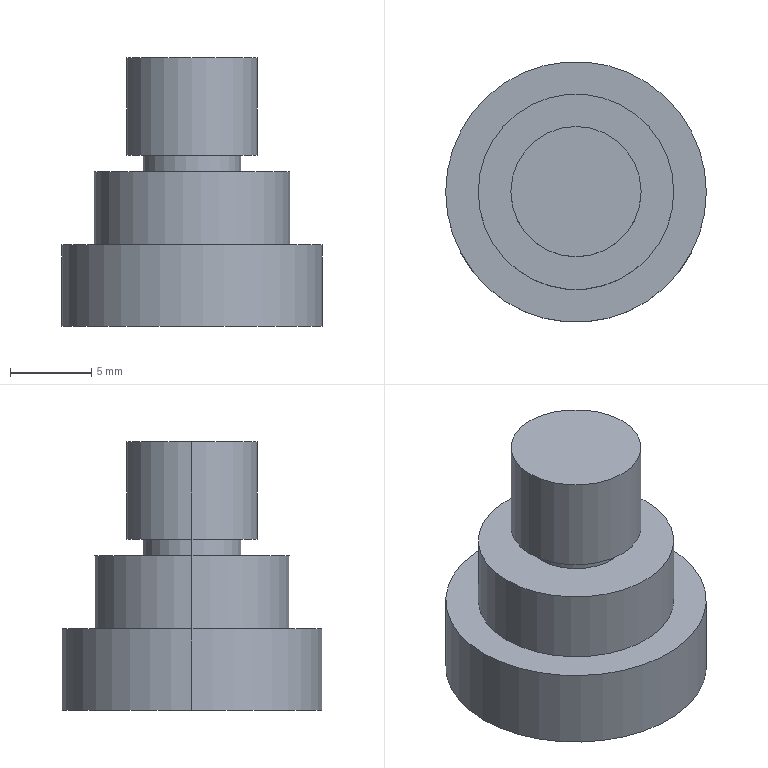Part | SolidWorks | features Revolution 1 | 1 solid | 13 faces | box 16 x 16 x 16.5 mm | volume 1844 mm3 | cylinder 8 | plane 5 | commonest cylinder face diameters 6 x2 8 x2 12 x2 16 x2
STEP:
#1=CARTESIAN_POINT('',(4.,0.,-6.));
#2=VERTEX_POINT('',#1);
#3=CARTESIAN_POINT('',(-4.,0.,-6.));
#4=VERTEX_POINT('',#3);
#5=CARTESIAN_POINT('',(0.,0.,-6.));
#6=DIRECTION('',(0.,0.,1.));
#7=DIRECTION('',(1.,0.,0.));
#8=AXIS2_PLACEMENT_3D('',#5,#6,#7);
#9=CIRCLE('',#8,4.);
#10=EDGE_CURVE('',#2,#4,#9,.T.);
#11=ORIENTED_EDGE('',*,*,#10,.T.);
#12=CARTESIAN_POINT('',(-4.,0.,0.));
#13=VERTEX_POINT('',#12);
#14=CARTESIAN_POINT('',(-4.,0.,0.));
#15=DIRECTION('',(0.,0.,1.));
#16=VECTOR('',#15,1000.);
#17=LINE('',#14,#16);
#18=EDGE_CURVE('',#4,#13,#17,.T.);
#19=ORIENTED_EDGE('',*,*,#18,.T.);
#20=CARTESIAN_POINT('',(4.,0.,0.));
#21=VERTEX_POINT('',#20);
#22=CARTESIAN_POINT('',(0.,0.,0.));
#23=DIRECTION('',(0.,0.,1.));
#24=DIRECTION('',(1.,0.,0.));
#25=AXIS2_PLACEMENT_3D('',#22,#23,#24);
#26=CIRCLE('',#25,4.);
#27=EDGE_CURVE('',#21,#13,#26,.T.);
#28=ORIENTED_EDGE('',*,*,#27,.F.);
#29=CARTESIAN_POINT('',(4.,0.,0.));
#30=DIRECTION('',(0.,0.,1.));
#31=VECTOR('',#30,1000.);
#32=LINE('',#29,#31);
#33=EDGE_CURVE('',#2,#21,#32,.T.);
#34=ORIENTED_EDGE('',*,*,#33,.F.);
#35=EDGE_LOOP('',(#11,#19,#28,#34));
#36=FACE_OUTER_BOUND('',#35,.T.);
#37=CARTESIAN_POINT('',(0.,0.,0.));
#38=DIRECTION('',(0.,0.,1.));
#39=DIRECTION('',(1.,0.,0.));
#40=AXIS2_PLACEMENT_3D('',#37,#38,#39);
#41=CYLINDRICAL_SURFACE('',#40,4.);
#42=ADVANCED_FACE('',(#36),#41,.T.);
#43=CARTESIAN_POINT('',(3.,0.,-7.));
#44=VERTEX_POINT('',#43);
#45=CARTESIAN_POINT('',(-3.,0.,-7.));
#46=VERTEX_POINT('',#45);
#47=CARTESIAN_POINT('',(0.,0.,-7.));
#48=DIRECTION('',(0.,0.,1.));
#49=DIRECTION('',(1.,0.,0.));
#50=AXIS2_PLACEMENT_3D('',#47,#48,#49);
#51=CIRCLE('',#50,3.);
#52=EDGE_CURVE('',#44,#46,#51,.T.);
#53=ORIENTED_EDGE('',*,*,#52,.T.);
#54=CARTESIAN_POINT('',(-3.,0.,-6.));
#55=VERTEX_POINT('',#54);
#56=CARTESIAN_POINT('',(-3.,0.,0.));
#57=DIRECTION('',(0.,0.,1.));
#58=VECTOR('',#57,1000.);
#59=LINE('',#56,#58);
#60=EDGE_CURVE('',#46,#55,#59,.T.);
#61=ORIENTED_EDGE('',*,*,#60,.T.);
#62=CARTESIAN_POINT('',(3.,0.,-6.));
#63=VERTEX_POINT('',#62);
#64=CARTESIAN_POINT('',(0.,0.,-6.));
#65=DIRECTION('',(0.,0.,1.));
#66=DIRECTION('',(1.,0.,0.));
#67=AXIS2_PLACEMENT_3D('',#64,#65,#66);
#68=CIRCLE('',#67,3.);
#69=EDGE_CURVE('',#63,#55,#68,.T.);
#70=ORIENTED_EDGE('',*,*,#69,.F.);
#71=CARTESIAN_POINT('',(3.,0.,0.));
#72=DIRECTION('',(0.,0.,1.));
#73=VECTOR('',#72,1000.);
#74=LINE('',#71,#73);
#75=EDGE_CURVE('',#44,#63,#74,.T.);
#76=ORIENTED_EDGE('',*,*,#75,.F.);
#77=EDGE_LOOP('',(#53,#61,#70,#76));
#78=FACE_OUTER_BOUND('',#77,.T.);
#79=CARTESIAN_POINT('',(0.,0.,0.));
#80=DIRECTION('',(0.,0.,1.));
#81=DIRECTION('',(1.,0.,0.));
#82=AXIS2_PLACEMENT_3D('',#79,#80,#81);
#83=CYLINDRICAL_SURFACE('',#82,3.);
#84=ADVANCED_FACE('',(#78),#83,.T.);
#85=CARTESIAN_POINT('',(6.,0.,-11.5));
#86=VERTEX_POINT('',#85);
#87=CARTESIAN_POINT('',(-6.,0.,-11.5));
#88=VERTEX_POINT('',#87);
#89=CARTESIAN_POINT('',(0.,0.,-11.5));
#90=DIRECTION('',(0.,0.,1.));
#91=DIRECTION('',(1.,0.,0.));
#92=AXIS2_PLACEMENT_3D('',#89,#90,#91);
#93=CIRCLE('',#92,6.);
#94=EDGE_CURVE('',#86,#88,#93,.T.);
#95=ORIENTED_EDGE('',*,*,#94,.T.);
#96=CARTESIAN_POINT('',(-6.,0.,-7.));
#97=VERTEX_POINT('',#96);
#98=CARTESIAN_POINT('',(-6.,0.,0.));
#99=DIRECTION('',(0.,0.,1.));
#100=VECTOR('',#99,1000.);
#101=LINE('',#98,#100);
#102=EDGE_CURVE('',#88,#97,#101,.T.);
#103=ORIENTED_EDGE('',*,*,#102,.T.);
#104=CARTESIAN_POINT('',(6.,0.,-7.));
#105=VERTEX_POINT('',#104);
#106=CARTESIAN_POINT('',(0.,0.,-7.));
#107=DIRECTION('',(0.,0.,1.));
#108=DIRECTION('',(1.,0.,0.));
#109=AXIS2_PLACEMENT_3D('',#106,#107,#108);
#110=CIRCLE('',#109,6.);
#111=EDGE_CURVE('',#105,#97,#110,.T.);
#112=ORIENTED_EDGE('',*,*,#111,.F.);
#113=CARTESIAN_POINT('',(6.,0.,0.));
#114=DIRECTION('',(0.,0.,1.));
#115=VECTOR('',#114,1000.);
#116=LINE('',#113,#115);
#117=EDGE_CURVE('',#86,#105,#116,.T.);
#118=ORIENTED_EDGE('',*,*,#117,.F.);
#119=EDGE_LOOP('',(#95,#103,#112,#118));
#120=FACE_OUTER_BOUND('',#119,.T.);
#121=CARTESIAN_POINT('',(0.,0.,0.));
#122=DIRECTION('',(0.,0.,1.));
#123=DIRECTION('',(1.,0.,0.));
#124=AXIS2_PLACEMENT_3D('',#121,#122,#123);
#125=CYLINDRICAL_SURFACE('',#124,6.);
#126=ADVANCED_FACE('',(#120),#125,.T.);
#127=CARTESIAN_POINT('',(8.,0.,-16.5));
#128=VERTEX_POINT('',#127);
#129=CARTESIAN_POINT('',(-8.,0.,-16.5));
#130=VERTEX_POINT('',#129);
#131=CARTESIAN_POINT('',(0.,0.,-16.5));
#132=DIRECTION('',(0.,0.,1.));
#133=DIRECTION('',(1.,0.,0.));
#134=AXIS2_PLACEMENT_3D('',#131,#132,#133);
#135=CIRCLE('',#134,8.);
#136=EDGE_CURVE('',#128,#130,#135,.T.);
#137=ORIENTED_EDGE('',*,*,#136,.T.);
#138=CARTESIAN_POINT('',(-8.,0.,-11.5));
#139=VERTEX_POINT('',#138);
#140=CARTESIAN_POINT('',(-8.,0.,0.));
#141=DIRECTION('',(0.,0.,1.));
#142=VECTOR('',#141,1000.);
#143=LINE('',#140,#142);
#144=EDGE_CURVE('',#130,#139,#143,.T.);
#145=ORIENTED_EDGE('',*,*,#144,.T.);
#146=CARTESIAN_POINT('',(8.,0.,-11.5));
#147=VERTEX_POINT('',#146);
#148=CARTESIAN_POINT('',(0.,0.,-11.5));
#149=DIRECTION('',(0.,0.,1.));
#150=DIRECTION('',(1.,0.,0.));
#151=AXIS2_PLACEMENT_3D('',#148,#149,#150);
#152=CIRCLE('',#151,8.);
#153=EDGE_CURVE('',#147,#139,#152,.T.);
#154=ORIENTED_EDGE('',*,*,#153,.F.);
#155=CARTESIAN_POINT('',(8.,0.,0.));
#156=DIRECTION('',(0.,0.,1.));
#157=VECTOR('',#156,1000.);
#158=LINE('',#155,#157);
#159=EDGE_CURVE('',#128,#147,#158,.T.);
#160=ORIENTED_EDGE('',*,*,#159,.F.);
#161=EDGE_LOOP('',(#137,#145,#154,#160));
#162=FACE_OUTER_BOUND('',#161,.T.);
#163=CARTESIAN_POINT('',(0.,0.,0.));
#164=DIRECTION('',(0.,0.,1.));
#165=DIRECTION('',(1.,0.,0.));
#166=AXIS2_PLACEMENT_3D('',#163,#164,#165);
#167=CYLINDRICAL_SURFACE('',#166,8.);
#168=ADVANCED_FACE('',(#162),#167,.T.);
#169=ORIENTED_EDGE('',*,*,#136,.F.);
#170=CARTESIAN_POINT('',(0.,0.,-16.5));
#171=DIRECTION('',(0.,0.,1.));
#172=DIRECTION('',(1.,0.,0.));
#173=AXIS2_PLACEMENT_3D('',#170,#171,#172);
#174=CIRCLE('',#173,8.);
#175=EDGE_CURVE('',#130,#128,#174,.T.);
#176=ORIENTED_EDGE('',*,*,#175,.F.);
#177=EDGE_LOOP('',(#169,#176));
#178=FACE_OUTER_BOUND('',#177,.T.);
#179=CARTESIAN_POINT('',(0.,0.,-16.5));
#180=DIRECTION('',(0.,0.,1.));
#181=DIRECTION('',(1.,0.,0.));
#182=AXIS2_PLACEMENT_3D('',#179,#180,#181);
#183=PLANE('',#182);
#184=ADVANCED_FACE('',(#178),#183,.F.);
#185=ORIENTED_EDGE('',*,*,#144,.F.);
#186=ORIENTED_EDGE('',*,*,#175,.T.);
#187=ORIENTED_EDGE('',*,*,#159,.T.);
#188=CARTESIAN_POINT('',(0.,0.,-11.5));
#189=DIRECTION('',(0.,0.,1.));
#190=DIRECTION('',(1.,0.,0.));
#191=AXIS2_PLACEMENT_3D('',#188,#189,#190);
#192=CIRCLE('',#191,8.);
#193=EDGE_CURVE('',#139,#147,#192,.T.);
#194=ORIENTED_EDGE('',*,*,#193,.F.);
#195=EDGE_LOOP('',(#185,#186,#187,#194));
#196=FACE_OUTER_BOUND('',#195,.T.);
#197=CARTESIAN_POINT('',(0.,0.,0.));
#198=DIRECTION('',(0.,0.,1.));
#199=DIRECTION('',(1.,0.,0.));
#200=AXIS2_PLACEMENT_3D('',#197,#198,#199);
#201=CYLINDRICAL_SURFACE('',#200,8.);
#202=ADVANCED_FACE('',(#196),#201,.T.);
#203=ORIENTED_EDGE('',*,*,#94,.F.);
#204=CARTESIAN_POINT('',(0.,0.,-11.5));
#205=DIRECTION('',(0.,0.,1.));
#206=DIRECTION('',(1.,0.,0.));
#207=AXIS2_PLACEMENT_3D('',#204,#205,#206);
#208=CIRCLE('',#207,6.);
#209=EDGE_CURVE('',#88,#86,#208,.T.);
#210=ORIENTED_EDGE('',*,*,#209,.F.);
#211=EDGE_LOOP('',(#203,#210));
#212=FACE_BOUND('',#211,.T.);
#213=ORIENTED_EDGE('',*,*,#153,.T.);
#214=ORIENTED_EDGE('',*,*,#193,.T.);
#215=EDGE_LOOP('',(#213,#214));
#216=FACE_OUTER_BOUND('',#215,.T.);
#217=CARTESIAN_POINT('',(0.,8.,-11.5));
#218=DIRECTION('',(0.,0.,-1.));
#219=DIRECTION('',(-1.,0.,0.));
#220=AXIS2_PLACEMENT_3D('',#217,#218,#219);
#221=PLANE('',#220);
#222=ADVANCED_FACE('',(#212,#216),#221,.F.);
#223=ORIENTED_EDGE('',*,*,#102,.F.);
#224=ORIENTED_EDGE('',*,*,#209,.T.);
#225=ORIENTED_EDGE('',*,*,#117,.T.);
#226=CARTESIAN_POINT('',(0.,0.,-7.));
#227=DIRECTION('',(0.,0.,1.));
#228=DIRECTION('',(1.,0.,0.));
#229=AXIS2_PLACEMENT_3D('',#226,#227,#228);
#230=CIRCLE('',#229,6.);
#231=EDGE_CURVE('',#97,#105,#230,.T.);
#232=ORIENTED_EDGE('',*,*,#231,.F.);
#233=EDGE_LOOP('',(#223,#224,#225,#232));
#234=FACE_OUTER_BOUND('',#233,.T.);
#235=CARTESIAN_POINT('',(0.,0.,0.));
#236=DIRECTION('',(0.,0.,1.));
#237=DIRECTION('',(1.,0.,0.));
#238=AXIS2_PLACEMENT_3D('',#235,#236,#237);
#239=CYLINDRICAL_SURFACE('',#238,6.);
#240=ADVANCED_FACE('',(#234),#239,.T.);
#241=ORIENTED_EDGE('',*,*,#52,.F.);
#242=CARTESIAN_POINT('',(0.,0.,-7.));
#243=DIRECTION('',(0.,0.,1.));
#244=DIRECTION('',(1.,0.,0.));
#245=AXIS2_PLACEMENT_3D('',#242,#243,#244);
#246=CIRCLE('',#245,3.);
#247=EDGE_CURVE('',#46,#44,#246,.T.);
#248=ORIENTED_EDGE('',*,*,#247,.F.);
#249=EDGE_LOOP('',(#241,#248));
#250=FACE_BOUND('',#249,.T.);
#251=ORIENTED_EDGE('',*,*,#111,.T.);
#252=ORIENTED_EDGE('',*,*,#231,.T.);
#253=EDGE_LOOP('',(#251,#252));
#254=FACE_OUTER_BOUND('',#253,.T.);
#255=CARTESIAN_POINT('',(0.,6.,-7.));
#256=DIRECTION('',(0.,0.,-1.));
#257=DIRECTION('',(-1.,0.,0.));
#258=AXIS2_PLACEMENT_3D('',#255,#256,#257);
#259=PLANE('',#258);
#260=ADVANCED_FACE('',(#250,#254),#259,.F.);
#261=ORIENTED_EDGE('',*,*,#60,.F.);
#262=ORIENTED_EDGE('',*,*,#247,.T.);
#263=ORIENTED_EDGE('',*,*,#75,.T.);
#264=CARTESIAN_POINT('',(0.,0.,-6.));
#265=DIRECTION('',(0.,0.,1.));
#266=DIRECTION('',(1.,0.,0.));
#267=AXIS2_PLACEMENT_3D('',#264,#265,#266);
#268=CIRCLE('',#267,3.);
#269=EDGE_CURVE('',#55,#63,#268,.T.);
#270=ORIENTED_EDGE('',*,*,#269,.F.);
#271=EDGE_LOOP('',(#261,#262,#263,#270));
#272=FACE_OUTER_BOUND('',#271,.T.);
#273=CARTESIAN_POINT('',(0.,0.,0.));
#274=DIRECTION('',(0.,0.,1.));
#275=DIRECTION('',(1.,0.,0.));
#276=AXIS2_PLACEMENT_3D('',#273,#274,#275);
#277=CYLINDRICAL_SURFACE('',#276,3.);
#278=ADVANCED_FACE('',(#272),#277,.T.);
#279=ORIENTED_EDGE('',*,*,#10,.F.);
#280=CARTESIAN_POINT('',(0.,0.,-6.));
#281=DIRECTION('',(0.,0.,1.));
#282=DIRECTION('',(1.,0.,0.));
#283=AXIS2_PLACEMENT_3D('',#280,#281,#282);
#284=CIRCLE('',#283,4.);
#285=EDGE_CURVE('',#4,#2,#284,.T.);
#286=ORIENTED_EDGE('',*,*,#285,.F.);
#287=EDGE_LOOP('',(#279,#286));
#288=FACE_OUTER_BOUND('',#287,.T.);
#289=ORIENTED_EDGE('',*,*,#69,.T.);
#290=ORIENTED_EDGE('',*,*,#269,.T.);
#291=EDGE_LOOP('',(#289,#290));
#292=FACE_BOUND('',#291,.T.);
#293=CARTESIAN_POINT('',(0.,3.,-6.));
#294=DIRECTION('',(0.,0.,1.));
#295=DIRECTION('',(1.,0.,0.));
#296=AXIS2_PLACEMENT_3D('',#293,#294,#295);
#297=PLANE('',#296);
#298=ADVANCED_FACE('',(#288,#292),#297,.F.);
#299=ORIENTED_EDGE('',*,*,#18,.F.);
#300=ORIENTED_EDGE('',*,*,#285,.T.);
#301=ORIENTED_EDGE('',*,*,#33,.T.);
#302=CARTESIAN_POINT('',(0.,0.,0.));
#303=DIRECTION('',(0.,0.,1.));
#304=DIRECTION('',(1.,0.,0.));
#305=AXIS2_PLACEMENT_3D('',#302,#303,#304);
#306=CIRCLE('',#305,4.);
#307=EDGE_CURVE('',#13,#21,#306,.T.);
#308=ORIENTED_EDGE('',*,*,#307,.F.);
#309=EDGE_LOOP('',(#299,#300,#301,#308));
#310=FACE_OUTER_BOUND('',#309,.T.);
#311=CARTESIAN_POINT('',(0.,0.,0.));
#312=DIRECTION('',(0.,0.,1.));
#313=DIRECTION('',(1.,0.,0.));
#314=AXIS2_PLACEMENT_3D('',#311,#312,#313);
#315=CYLINDRICAL_SURFACE('',#314,4.);
#316=ADVANCED_FACE('',(#310),#315,.T.);
#317=ORIENTED_EDGE('',*,*,#27,.T.);
#318=ORIENTED_EDGE('',*,*,#307,.T.);
#319=EDGE_LOOP('',(#317,#318));
#320=FACE_OUTER_BOUND('',#319,.T.);
#321=CARTESIAN_POINT('',(0.,4.,0.));
#322=DIRECTION('',(0.,0.,-1.));
#323=DIRECTION('',(-1.,0.,0.));
#324=AXIS2_PLACEMENT_3D('',#321,#322,#323);
#325=PLANE('',#324);
#326=ADVANCED_FACE('',(#320),#325,.F.);
#327=CLOSED_SHELL('',(#42,#84,#126,#168,#184,#202,#222,#240,#260,#278,#298,#316,#326));
#328=MANIFOLD_SOLID_BREP('',#327);
#329=CARTESIAN_POINT('',(0.,0.,0.));
#330=DIRECTION('',(0.,0.,1.));
#331=DIRECTION('',(1.,0.,0.));
#332=AXIS2_PLACEMENT_3D('',#329,#330,#331);
#333=(LENGTH_UNIT()NAMED_UNIT(*)SI_UNIT(.MILLI.,.METRE.));
#334=UNCERTAINTY_MEASURE_WITH_UNIT(LENGTH_MEASURE(0.00001),#333,'','');
#335=(NAMED_UNIT(*)PLANE_ANGLE_UNIT()SI_UNIT($,.RADIAN.));
#336=(NAMED_UNIT(*)SI_UNIT($,.STERADIAN.)SOLID_ANGLE_UNIT());
#337=(GEOMETRIC_REPRESENTATION_CONTEXT(3)GLOBAL_UNCERTAINTY_ASSIGNED_CONTEXT((#334))GLOBAL_UNIT_ASSIGNED_CONTEXT((#333,#335,#336))REPRESENTATION_CONTEXT('',''));
#338=ADVANCED_BREP_SHAPE_REPRESENTATION('',(#328,#332),#337);